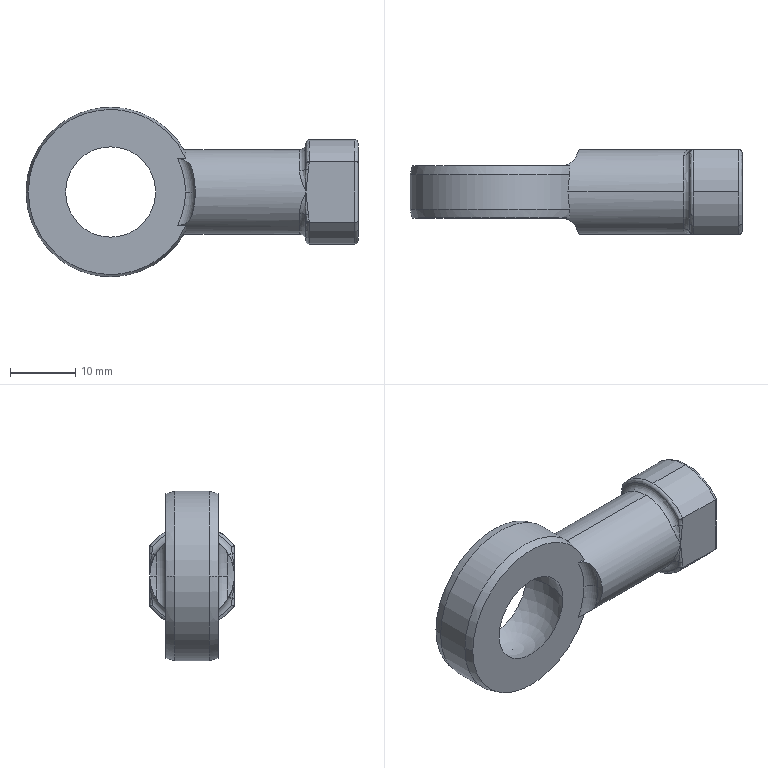Part | STEP file | M8 Body Female | 1 solid | 54 faces | box 51 x 13 x 26 mm | volume 5699 mm3 | cylinder 17 | torus 12 | spline 12 | sphere 6 | plane 5 | cone 2 | commonest cylinder face diameters 1 x6 26 x4 16 x3 6.8 x2 13 x2